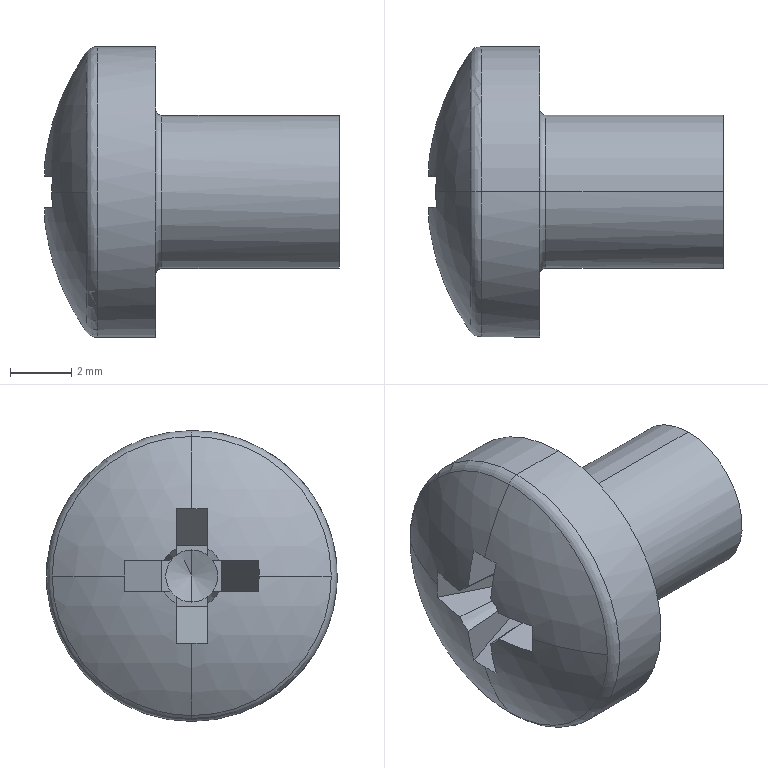Part | STEP file | PN_0035_Default<As Machined> | 1 solid | 36 faces | box 9.632 x 9.5 x 9.5 mm | volume 311.012 mm3 | plane 18 | cone 6 | sphere 4 | torus 4 | cylinder 4 | commonest cylinder face diameters 5 x2 9.5 x2